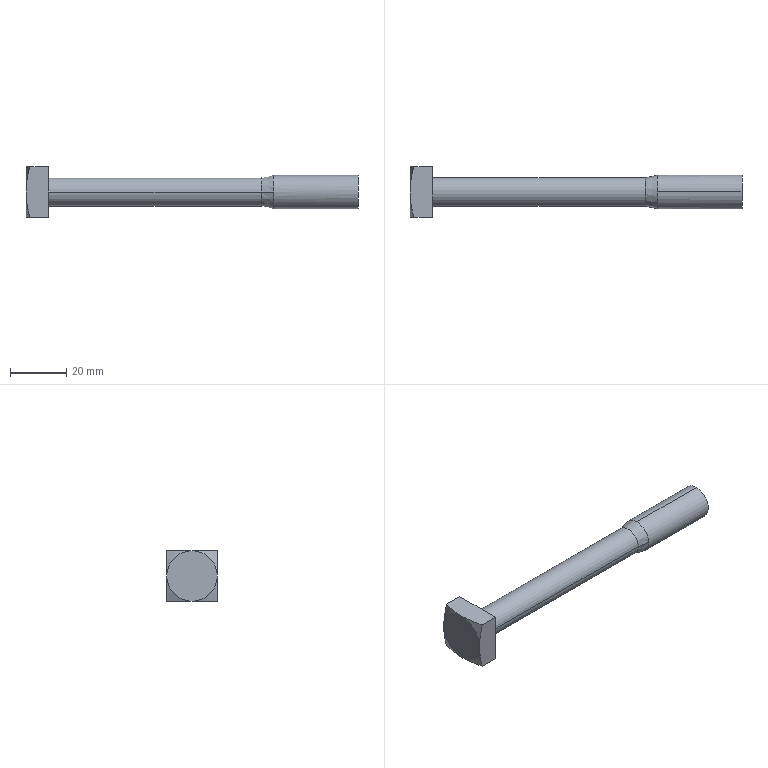Part | SolidWorks | features RevCut 3, Boss 1, Extrusion 1, LPattern 1 | 1 solid | 17 faces | box 118 x 18 x 18 mm | volume 12442 mm3 | plane 7 | cone 6 | cylinder 4 | commonest cylinder face diameters 10.106 x2 12 x2
STEP:
#1=CARTESIAN_POINT('',(118.,0.,-6.));
#2=VERTEX_POINT('',#1);
#3=CARTESIAN_POINT('',(118.,0.,6.));
#4=VERTEX_POINT('',#3);
#5=CARTESIAN_POINT('',(118.,0.,0.));
#6=DIRECTION('',(1.,0.,0.));
#7=DIRECTION('',(0.,0.,-1.));
#8=AXIS2_PLACEMENT_3D('',#5,#6,#7);
#9=CIRCLE('',#8,6.);
#10=EDGE_CURVE('',#2,#4,#9,.T.);
#11=ORIENTED_EDGE('',*,*,#10,.F.);
#12=CARTESIAN_POINT('',(88.,0.,-6.));
#13=VERTEX_POINT('',#12);
#14=CARTESIAN_POINT('',(118.,0.,-6.));
#15=DIRECTION('',(-1.,0.,0.));
#16=VECTOR('',#15,1000.);
#17=LINE('',#14,#16);
#18=EDGE_CURVE('',#2,#13,#17,.T.);
#19=ORIENTED_EDGE('',*,*,#18,.T.);
#20=CARTESIAN_POINT('',(88.,6.,0.));
#21=VERTEX_POINT('',#20);
#22=CARTESIAN_POINT('',(88.,0.,0.));
#23=DIRECTION('',(-1.,0.,0.));
#24=DIRECTION('',(0.,-1.,0.));
#25=AXIS2_PLACEMENT_3D('',#22,#23,#24);
#26=CIRCLE('',#25,6.);
#27=EDGE_CURVE('',#21,#13,#26,.T.);
#28=ORIENTED_EDGE('',*,*,#27,.F.);
#29=CARTESIAN_POINT('',(88.,0.,6.));
#30=VERTEX_POINT('',#29);
#31=CARTESIAN_POINT('',(88.,0.,0.));
#32=DIRECTION('',(-1.,0.,0.));
#33=DIRECTION('',(0.,-1.,0.));
#34=AXIS2_PLACEMENT_3D('',#31,#32,#33);
#35=CIRCLE('',#34,6.);
#36=EDGE_CURVE('',#30,#21,#35,.T.);
#37=ORIENTED_EDGE('',*,*,#36,.F.);
#38=CARTESIAN_POINT('',(118.,0.,6.));
#39=DIRECTION('',(-1.,0.,0.));
#40=VECTOR('',#39,1000.);
#41=LINE('',#38,#40);
#42=EDGE_CURVE('',#4,#30,#41,.T.);
#43=ORIENTED_EDGE('',*,*,#42,.F.);
#44=EDGE_LOOP('',(#11,#19,#28,#37,#43));
#45=FACE_OUTER_BOUND('',#44,.T.);
#46=CARTESIAN_POINT('',(118.,0.,0.));
#47=DIRECTION('',(-1.,0.,0.));
#48=DIRECTION('',(0.,0.,1.));
#49=AXIS2_PLACEMENT_3D('',#46,#47,#48);
#50=CYLINDRICAL_SURFACE('',#49,6.);
#51=ADVANCED_FACE('',(#45),#50,.T.);
#52=CARTESIAN_POINT('',(83.7,-5.053,0.));
#53=VERTEX_POINT('',#52);
#54=CARTESIAN_POINT('',(83.7,5.053,0.));
#55=VERTEX_POINT('',#54);
#56=CARTESIAN_POINT('',(83.7,0.,0.));
#57=DIRECTION('',(-1.,0.,0.));
#58=DIRECTION('',(0.,-1.,0.));
#59=AXIS2_PLACEMENT_3D('',#56,#57,#58);
#60=CIRCLE('',#59,5.053);
#61=EDGE_CURVE('',#53,#55,#60,.T.);
#62=ORIENTED_EDGE('',*,*,#61,.T.);
#63=CARTESIAN_POINT('',(8.,5.053,0.));
#64=VERTEX_POINT('',#63);
#65=CARTESIAN_POINT('',(-3.791,5.053,0.));
#66=DIRECTION('',(-1.,0.,0.));
#67=VECTOR('',#66,1000.);
#68=LINE('',#65,#67);
#69=EDGE_CURVE('',#55,#64,#68,.T.);
#70=ORIENTED_EDGE('',*,*,#69,.T.);
#71=CARTESIAN_POINT('',(8.,-5.053,0.));
#72=VERTEX_POINT('',#71);
#73=CARTESIAN_POINT('',(8.,0.,0.));
#74=DIRECTION('',(-1.,0.,0.));
#75=DIRECTION('',(0.,-1.,0.));
#76=AXIS2_PLACEMENT_3D('',#73,#74,#75);
#77=CIRCLE('',#76,5.053);
#78=EDGE_CURVE('',#72,#64,#77,.T.);
#79=ORIENTED_EDGE('',*,*,#78,.F.);
#80=CARTESIAN_POINT('',(-3.791,-5.053,0.));
#81=DIRECTION('',(-1.,0.,0.));
#82=VECTOR('',#81,1000.);
#83=LINE('',#80,#82);
#84=EDGE_CURVE('',#53,#72,#83,.T.);
#85=ORIENTED_EDGE('',*,*,#84,.F.);
#86=EDGE_LOOP('',(#62,#70,#79,#85));
#87=FACE_OUTER_BOUND('',#86,.T.);
#88=CARTESIAN_POINT('',(-3.791,0.,0.));
#89=DIRECTION('',(-1.,0.,0.));
#90=DIRECTION('',(0.,-1.,0.));
#91=AXIS2_PLACEMENT_3D('',#88,#89,#90);
#92=CYLINDRICAL_SURFACE('',#91,5.053);
#93=ADVANCED_FACE('',(#87),#92,.T.);
#94=ORIENTED_EDGE('',*,*,#61,.F.);
#95=CARTESIAN_POINT('',(88.,-6.,0.));
#96=VERTEX_POINT('',#95);
#97=CARTESIAN_POINT('',(88.,-6.,0.));
#98=DIRECTION('',(0.9766,-0.2151,0.));
#99=VECTOR('',#98,1000.);
#100=LINE('',#97,#99);
#101=EDGE_CURVE('',#53,#96,#100,.T.);
#102=ORIENTED_EDGE('',*,*,#101,.T.);
#103=CARTESIAN_POINT('',(88.,0.,0.));
#104=DIRECTION('',(-1.,0.,0.));
#105=DIRECTION('',(0.,-1.,0.));
#106=AXIS2_PLACEMENT_3D('',#103,#104,#105);
#107=CIRCLE('',#106,6.);
#108=EDGE_CURVE('',#96,#30,#107,.T.);
#109=ORIENTED_EDGE('',*,*,#108,.T.);
#110=ORIENTED_EDGE('',*,*,#36,.T.);
#111=CARTESIAN_POINT('',(88.,6.,0.));
#112=DIRECTION('',(0.9766,0.2151,0.));
#113=VECTOR('',#112,1000.);
#114=LINE('',#111,#113);
#115=EDGE_CURVE('',#55,#21,#114,.T.);
#116=ORIENTED_EDGE('',*,*,#115,.F.);
#117=EDGE_LOOP('',(#94,#102,#109,#110,#116));
#118=FACE_OUTER_BOUND('',#117,.T.);
#119=CARTESIAN_POINT('',(88.,0.,0.));
#120=DIRECTION('',(1.,0.,0.));
#121=DIRECTION('',(0.,1.,0.));
#122=AXIS2_PLACEMENT_3D('',#119,#120,#121);
#123=CONICAL_SURFACE('',#122,6.,0.2168);
#124=ADVANCED_FACE('',(#118),#123,.T.);
#125=CARTESIAN_POINT('',(8.,9.,9.));
#126=VERTEX_POINT('',#125);
#127=CARTESIAN_POINT('',(8.,-9.,9.));
#128=VERTEX_POINT('',#127);
#129=CARTESIAN_POINT('',(8.,9.,9.));
#130=DIRECTION('',(0.,-1.,0.));
#131=VECTOR('',#130,1000.);
#132=LINE('',#129,#131);
#133=EDGE_CURVE('',#126,#128,#132,.T.);
#134=ORIENTED_EDGE('',*,*,#133,.T.);
#135=CARTESIAN_POINT('',(8.,-9.,-9.));
#136=VERTEX_POINT('',#135);
#137=CARTESIAN_POINT('',(8.,-9.,9.));
#138=DIRECTION('',(0.,0.,-1.));
#139=VECTOR('',#138,1000.);
#140=LINE('',#137,#139);
#141=EDGE_CURVE('',#128,#136,#140,.T.);
#142=ORIENTED_EDGE('',*,*,#141,.T.);
#143=CARTESIAN_POINT('',(8.,9.,-9.));
#144=VERTEX_POINT('',#143);
#145=CARTESIAN_POINT('',(8.,9.,-9.));
#146=DIRECTION('',(0.,1.,0.));
#147=VECTOR('',#146,1000.);
#148=LINE('',#145,#147);
#149=EDGE_CURVE('',#136,#144,#148,.T.);
#150=ORIENTED_EDGE('',*,*,#149,.T.);
#151=CARTESIAN_POINT('',(8.,9.,9.));
#152=DIRECTION('',(0.,0.,1.));
#153=VECTOR('',#152,1000.);
#154=LINE('',#151,#153);
#155=EDGE_CURVE('',#144,#126,#154,.T.);
#156=ORIENTED_EDGE('',*,*,#155,.T.);
#157=EDGE_LOOP('',(#134,#142,#150,#156));
#158=FACE_OUTER_BOUND('',#157,.T.);
#159=ORIENTED_EDGE('',*,*,#78,.T.);
#160=CARTESIAN_POINT('',(8.,0.,0.));
#161=DIRECTION('',(-1.,0.,0.));
#162=DIRECTION('',(0.,-1.,0.));
#163=AXIS2_PLACEMENT_3D('',#160,#161,#162);
#164=CIRCLE('',#163,5.053);
#165=EDGE_CURVE('',#64,#72,#164,.T.);
#166=ORIENTED_EDGE('',*,*,#165,.T.);
#167=EDGE_LOOP('',(#159,#166));
#168=FACE_BOUND('',#167,.T.);
#169=CARTESIAN_POINT('',(8.,-9.,9.));
#170=DIRECTION('',(1.,0.,0.));
#171=DIRECTION('',(0.,0.,-1.));
#172=AXIS2_PLACEMENT_3D('',#169,#170,#171);
#173=PLANE('',#172);
#174=ADVANCED_FACE('',(#158,#168),#173,.T.);
#175=CARTESIAN_POINT('',(1.357,-9.,9.));
#176=VERTEX_POINT('',#175);
#177=CARTESIAN_POINT('',(0.,0.,9.));
#178=VERTEX_POINT('',#177);
#179=CARTESIAN_POINT('',(1.357,-9.,9.));
#180=CARTESIAN_POINT('',(0.9754,-7.518,9.));
#181=CARTESIAN_POINT('',(0.6345,-6.018,9.));
#182=CARTESIAN_POINT('',(0.1443,-3.016,9.));
#183=CARTESIAN_POINT('',(0.,-1.511,9.));
#184=CARTESIAN_POINT('',(0.,0.,9.));
#185=B_SPLINE_CURVE_WITH_KNOTS('',3,(#179,#180,#181,#182,#183,#184),.UNSPECIFIED.,.F.,.F.,(4,2,4),(0.009265,0.01385,0.01844),.UNSPECIFIED.);
#186=EDGE_CURVE('',#176,#178,#185,.T.);
#187=ORIENTED_EDGE('',*,*,#186,.F.);
#188=CARTESIAN_POINT('',(8.,-9.,9.));
#189=DIRECTION('',(-1.,0.,0.));
#190=VECTOR('',#189,1000.);
#191=LINE('',#188,#190);
#192=EDGE_CURVE('',#128,#176,#191,.T.);
#193=ORIENTED_EDGE('',*,*,#192,.F.);
#194=ORIENTED_EDGE('',*,*,#133,.F.);
#195=CARTESIAN_POINT('',(1.357,9.,9.));
#196=VERTEX_POINT('',#195);
#197=CARTESIAN_POINT('',(8.,9.,9.));
#198=DIRECTION('',(-1.,0.,0.));
#199=VECTOR('',#198,1000.);
#200=LINE('',#197,#199);
#201=EDGE_CURVE('',#126,#196,#200,.T.);
#202=ORIENTED_EDGE('',*,*,#201,.T.);
#203=CARTESIAN_POINT('',(0.,0.,9.));
#204=CARTESIAN_POINT('',(0.,0.7525,9.));
#205=CARTESIAN_POINT('',(0.03485,1.506,9.));
#206=CARTESIAN_POINT('',(0.1688,3.017,9.));
#207=CARTESIAN_POINT('',(0.2678,3.774,9.));
#208=CARTESIAN_POINT('',(0.6392,6.043,9.));
#209=CARTESIAN_POINT('',(0.978,7.528,9.));
#210=CARTESIAN_POINT('',(1.357,9.,9.));
#211=B_SPLINE_CURVE_WITH_KNOTS('',3,(#203,#204,#205,#206,#207,#208,#209,#210),.UNSPECIFIED.,.F.,.F.,(4,2,2,4),(0.01844,0.02073,0.02302,0.02759),.UNSPECIFIED.);
#212=EDGE_CURVE('',#178,#196,#211,.T.);
#213=ORIENTED_EDGE('',*,*,#212,.F.);
#214=EDGE_LOOP('',(#187,#193,#194,#202,#213));
#215=FACE_OUTER_BOUND('',#214,.T.);
#216=CARTESIAN_POINT('',(8.,9.,9.));
#217=DIRECTION('',(0.,0.,-1.));
#218=DIRECTION('',(-1.,0.,0.));
#219=AXIS2_PLACEMENT_3D('',#216,#217,#218);
#220=PLANE('',#219);
#221=ADVANCED_FACE('',(#215),#220,.F.);
#222=CARTESIAN_POINT('',(1.357,-9.,-9.));
#223=VERTEX_POINT('',#222);
#224=CARTESIAN_POINT('',(0.,-9.,0.));
#225=VERTEX_POINT('',#224);
#226=CARTESIAN_POINT('',(1.357,-9.,-9.));
#227=CARTESIAN_POINT('',(0.9754,-9.,-7.518));
#228=CARTESIAN_POINT('',(0.6345,-9.,-6.018));
#229=CARTESIAN_POINT('',(0.1443,-9.,-3.016));
#230=CARTESIAN_POINT('',(0.,-9.,-1.511));
#231=CARTESIAN_POINT('',(0.,-9.,0.));
#232=B_SPLINE_CURVE_WITH_KNOTS('',3,(#226,#227,#228,#229,#230,#231),.UNSPECIFIED.,.F.,.F.,(4,2,4),(0.009265,0.01385,0.01844),.UNSPECIFIED.);
#233=EDGE_CURVE('',#223,#225,#232,.T.);
#234=ORIENTED_EDGE('',*,*,#233,.F.);
#235=CARTESIAN_POINT('',(8.,-9.,-9.));
#236=DIRECTION('',(-1.,0.,0.));
#237=VECTOR('',#236,1000.);
#238=LINE('',#235,#237);
#239=EDGE_CURVE('',#136,#223,#238,.T.);
#240=ORIENTED_EDGE('',*,*,#239,.F.);
#241=ORIENTED_EDGE('',*,*,#141,.F.);
#242=ORIENTED_EDGE('',*,*,#192,.T.);
#243=CARTESIAN_POINT('',(0.,-9.,0.));
#244=CARTESIAN_POINT('',(0.,-9.,0.7525));
#245=CARTESIAN_POINT('',(0.03485,-9.,1.506));
#246=CARTESIAN_POINT('',(0.1688,-9.,3.017));
#247=CARTESIAN_POINT('',(0.2678,-9.,3.774));
#248=CARTESIAN_POINT('',(0.6392,-9.,6.043));
#249=CARTESIAN_POINT('',(0.978,-9.,7.528));
#250=CARTESIAN_POINT('',(1.357,-9.,9.));
#251=B_SPLINE_CURVE_WITH_KNOTS('',3,(#243,#244,#245,#246,#247,#248,#249,#250),.UNSPECIFIED.,.F.,.F.,(4,2,2,4),(0.01844,0.02073,0.02302,0.02759),.UNSPECIFIED.);
#252=EDGE_CURVE('',#225,#176,#251,.T.);
#253=ORIENTED_EDGE('',*,*,#252,.F.);
#254=EDGE_LOOP('',(#234,#240,#241,#242,#253));
#255=FACE_OUTER_BOUND('',#254,.T.);
#256=CARTESIAN_POINT('',(8.,-9.,9.));
#257=DIRECTION('',(0.,1.,0.));
#258=DIRECTION('',(0.,0.,1.));
#259=AXIS2_PLACEMENT_3D('',#256,#257,#258);
#260=PLANE('',#259);
#261=ADVANCED_FACE('',(#255),#260,.F.);
#262=CARTESIAN_POINT('',(1.357,9.,-9.));
#263=VERTEX_POINT('',#262);
#264=CARTESIAN_POINT('',(0.,0.,-9.));
#265=VERTEX_POINT('',#264);
#266=CARTESIAN_POINT('',(1.357,9.,-9.));
#267=CARTESIAN_POINT('',(0.978,7.528,-9.));
#268=CARTESIAN_POINT('',(0.6392,6.043,-9.));
#269=CARTESIAN_POINT('',(0.2678,3.774,-9.));
#270=CARTESIAN_POINT('',(0.1688,3.017,-9.));
#271=CARTESIAN_POINT('',(0.03485,1.506,-9.));
#272=CARTESIAN_POINT('',(0.,0.7525,-9.));
#273=CARTESIAN_POINT('',(0.,0.,-9.));
#274=B_SPLINE_CURVE_WITH_KNOTS('',3,(#266,#267,#268,#269,#270,#271,#272,#273),.UNSPECIFIED.,.F.,.F.,(4,2,2,4),(0.02832,0.03288,0.03516,0.03743),.UNSPECIFIED.);
#275=EDGE_CURVE('',#263,#265,#274,.T.);
#276=ORIENTED_EDGE('',*,*,#275,.F.);
#277=CARTESIAN_POINT('',(8.,9.,-9.));
#278=DIRECTION('',(-1.,0.,0.));
#279=VECTOR('',#278,1000.);
#280=LINE('',#277,#279);
#281=EDGE_CURVE('',#144,#263,#280,.T.);
#282=ORIENTED_EDGE('',*,*,#281,.F.);
#283=ORIENTED_EDGE('',*,*,#149,.F.);
#284=ORIENTED_EDGE('',*,*,#239,.T.);
#285=CARTESIAN_POINT('',(0.,0.,-9.));
#286=CARTESIAN_POINT('',(0.,-1.511,-9.));
#287=CARTESIAN_POINT('',(0.1443,-3.016,-9.));
#288=CARTESIAN_POINT('',(0.6345,-6.018,-9.));
#289=CARTESIAN_POINT('',(0.9754,-7.518,-9.));
#290=CARTESIAN_POINT('',(1.357,-9.,-9.));
#291=B_SPLINE_CURVE_WITH_KNOTS('',3,(#285,#286,#287,#288,#289,#290),.UNSPECIFIED.,.F.,.F.,(4,2,4),(0.03743,0.042,0.04658),.UNSPECIFIED.);
#292=EDGE_CURVE('',#265,#223,#291,.T.);
#293=ORIENTED_EDGE('',*,*,#292,.F.);
#294=EDGE_LOOP('',(#276,#282,#283,#284,#293));
#295=FACE_OUTER_BOUND('',#294,.T.);
#296=CARTESIAN_POINT('',(8.,9.,-9.));
#297=DIRECTION('',(0.,0.,1.));
#298=DIRECTION('',(0.,-1.,0.));
#299=AXIS2_PLACEMENT_3D('',#296,#297,#298);
#300=PLANE('',#299);
#301=ADVANCED_FACE('',(#295),#300,.F.);
#302=CARTESIAN_POINT('',(0.,9.,0.));
#303=VERTEX_POINT('',#302);
#304=CARTESIAN_POINT('',(1.357,9.,9.));
#305=CARTESIAN_POINT('',(0.978,9.,7.528));
#306=CARTESIAN_POINT('',(0.6392,9.,6.043));
#307=CARTESIAN_POINT('',(0.2678,9.,3.774));
#308=CARTESIAN_POINT('',(0.1688,9.,3.017));
#309=CARTESIAN_POINT('',(0.03485,9.,1.506));
#310=CARTESIAN_POINT('',(0.,9.,0.7525));
#311=CARTESIAN_POINT('',(0.,9.,0.));
#312=B_SPLINE_CURVE_WITH_KNOTS('',3,(#304,#305,#306,#307,#308,#309,#310,#311),.UNSPECIFIED.,.F.,.F.,(4,2,2,4),(0.02832,0.03288,0.03516,0.03743),.UNSPECIFIED.);
#313=EDGE_CURVE('',#196,#303,#312,.T.);
#314=ORIENTED_EDGE('',*,*,#313,.F.);
#315=ORIENTED_EDGE('',*,*,#201,.F.);
#316=ORIENTED_EDGE('',*,*,#155,.F.);
#317=ORIENTED_EDGE('',*,*,#281,.T.);
#318=CARTESIAN_POINT('',(0.,9.,0.));
#319=CARTESIAN_POINT('',(0.,9.,-1.511));
#320=CARTESIAN_POINT('',(0.1443,9.,-3.016));
#321=CARTESIAN_POINT('',(0.6345,9.,-6.018));
#322=CARTESIAN_POINT('',(0.9754,9.,-7.518));
#323=CARTESIAN_POINT('',(1.357,9.,-9.));
#324=B_SPLINE_CURVE_WITH_KNOTS('',3,(#318,#319,#320,#321,#322,#323),.UNSPECIFIED.,.F.,.F.,(4,2,4),(0.03743,0.042,0.04658),.UNSPECIFIED.);
#325=EDGE_CURVE('',#303,#263,#324,.T.);
#326=ORIENTED_EDGE('',*,*,#325,.F.);
#327=EDGE_LOOP('',(#314,#315,#316,#317,#326));
#328=FACE_OUTER_BOUND('',#327,.T.);
#329=CARTESIAN_POINT('',(8.,9.,9.));
#330=DIRECTION('',(0.,-1.,0.));
#331=DIRECTION('',(0.,0.,-1.));
#332=AXIS2_PLACEMENT_3D('',#329,#330,#331);
#333=PLANE('',#332);
#334=ADVANCED_FACE('',(#328),#333,.F.);
#335=ORIENTED_EDGE('',*,*,#233,.T.);
#336=CARTESIAN_POINT('',(0.,0.,0.));
#337=DIRECTION('',(1.,0.,0.));
#338=DIRECTION('',(0.,0.,-1.));
#339=AXIS2_PLACEMENT_3D('',#336,#337,#338);
#340=CIRCLE('',#339,9.);
#341=EDGE_CURVE('',#225,#265,#340,.T.);
#342=ORIENTED_EDGE('',*,*,#341,.T.);
#343=ORIENTED_EDGE('',*,*,#292,.T.);
#344=EDGE_LOOP('',(#335,#342,#343));
#345=FACE_OUTER_BOUND('',#344,.T.);
#346=CARTESIAN_POINT('',(1.357,0.,0.));
#347=DIRECTION('',(1.,0.,0.));
#348=DIRECTION('',(0.,0.,-1.));
#349=AXIS2_PLACEMENT_3D('',#346,#347,#348);
#350=CONICAL_SURFACE('',#349,12.728,1.222);
#351=ADVANCED_FACE('',(#345),#350,.T.);
#352=ORIENTED_EDGE('',*,*,#252,.T.);
#353=ORIENTED_EDGE('',*,*,#186,.T.);
#354=CARTESIAN_POINT('',(0.,0.,0.));
#355=DIRECTION('',(1.,0.,0.));
#356=DIRECTION('',(0.,0.,-1.));
#357=AXIS2_PLACEMENT_3D('',#354,#355,#356);
#358=CIRCLE('',#357,9.);
#359=EDGE_CURVE('',#178,#225,#358,.T.);
#360=ORIENTED_EDGE('',*,*,#359,.T.);
#361=EDGE_LOOP('',(#352,#353,#360));
#362=FACE_OUTER_BOUND('',#361,.T.);
#363=CARTESIAN_POINT('',(1.357,0.,0.));
#364=DIRECTION('',(1.,0.,0.));
#365=DIRECTION('',(0.,0.,-1.));
#366=AXIS2_PLACEMENT_3D('',#363,#364,#365);
#367=CONICAL_SURFACE('',#366,12.728,1.222);
#368=ADVANCED_FACE('',(#362),#367,.T.);
#369=ORIENTED_EDGE('',*,*,#212,.T.);
#370=ORIENTED_EDGE('',*,*,#313,.T.);
#371=CARTESIAN_POINT('',(0.,0.,0.));
#372=DIRECTION('',(1.,0.,0.));
#373=DIRECTION('',(0.,0.,-1.));
#374=AXIS2_PLACEMENT_3D('',#371,#372,#373);
#375=CIRCLE('',#374,9.);
#376=EDGE_CURVE('',#303,#178,#375,.T.);
#377=ORIENTED_EDGE('',*,*,#376,.T.);
#378=EDGE_LOOP('',(#369,#370,#377));
#379=FACE_OUTER_BOUND('',#378,.T.);
#380=CARTESIAN_POINT('',(1.357,0.,0.));
#381=DIRECTION('',(1.,0.,0.));
#382=DIRECTION('',(0.,0.,-1.));
#383=AXIS2_PLACEMENT_3D('',#380,#381,#382);
#384=CONICAL_SURFACE('',#383,12.728,1.222);
#385=ADVANCED_FACE('',(#379),#384,.T.);
#386=ORIENTED_EDGE('',*,*,#275,.T.);
#387=CARTESIAN_POINT('',(0.,0.,0.));
#388=DIRECTION('',(1.,0.,0.));
#389=DIRECTION('',(0.,0.,-1.));
#390=AXIS2_PLACEMENT_3D('',#387,#388,#389);
#391=CIRCLE('',#390,9.);
#392=EDGE_CURVE('',#265,#303,#391,.T.);
#393=ORIENTED_EDGE('',*,*,#392,.T.);
#394=ORIENTED_EDGE('',*,*,#325,.T.);
#395=EDGE_LOOP('',(#386,#393,#394));
#396=FACE_OUTER_BOUND('',#395,.T.);
#397=CARTESIAN_POINT('',(1.357,0.,0.));
#398=DIRECTION('',(1.,0.,0.));
#399=DIRECTION('',(0.,0.,-1.));
#400=AXIS2_PLACEMENT_3D('',#397,#398,#399);
#401=CONICAL_SURFACE('',#400,12.728,1.222);
#402=ADVANCED_FACE('',(#396),#401,.T.);
#403=ORIENTED_EDGE('',*,*,#392,.F.);
#404=ORIENTED_EDGE('',*,*,#341,.F.);
#405=ORIENTED_EDGE('',*,*,#359,.F.);
#406=ORIENTED_EDGE('',*,*,#376,.F.);
#407=EDGE_LOOP('',(#403,#404,#405,#406));
#408=FACE_OUTER_BOUND('',#407,.T.);
#409=CARTESIAN_POINT('',(0.,-9.,9.));
#410=DIRECTION('',(1.,0.,0.));
#411=DIRECTION('',(0.,0.,-1.));
#412=AXIS2_PLACEMENT_3D('',#409,#410,#411);
#413=PLANE('',#412);
#414=ADVANCED_FACE('',(#408),#413,.F.);
#415=ORIENTED_EDGE('',*,*,#101,.F.);
#416=CARTESIAN_POINT('',(83.7,0.,0.));
#417=DIRECTION('',(-1.,0.,0.));
#418=DIRECTION('',(0.,-1.,0.));
#419=AXIS2_PLACEMENT_3D('',#416,#417,#418);
#420=CIRCLE('',#419,5.053);
#421=EDGE_CURVE('',#55,#53,#420,.T.);
#422=ORIENTED_EDGE('',*,*,#421,.F.);
#423=ORIENTED_EDGE('',*,*,#115,.T.);
#424=ORIENTED_EDGE('',*,*,#27,.T.);
#425=CARTESIAN_POINT('',(88.,0.,0.));
#426=DIRECTION('',(-1.,0.,0.));
#427=DIRECTION('',(0.,-1.,0.));
#428=AXIS2_PLACEMENT_3D('',#425,#426,#427);
#429=CIRCLE('',#428,6.);
#430=EDGE_CURVE('',#13,#96,#429,.T.);
#431=ORIENTED_EDGE('',*,*,#430,.T.);
#432=EDGE_LOOP('',(#415,#422,#423,#424,#431));
#433=FACE_OUTER_BOUND('',#432,.T.);
#434=CARTESIAN_POINT('',(88.,0.,0.));
#435=DIRECTION('',(1.,0.,0.));
#436=DIRECTION('',(0.,1.,0.));
#437=AXIS2_PLACEMENT_3D('',#434,#435,#436);
#438=CONICAL_SURFACE('',#437,6.,0.2168);
#439=ADVANCED_FACE('',(#433),#438,.T.);
#440=ORIENTED_EDGE('',*,*,#69,.F.);
#441=ORIENTED_EDGE('',*,*,#421,.T.);
#442=ORIENTED_EDGE('',*,*,#84,.T.);
#443=ORIENTED_EDGE('',*,*,#165,.F.);
#444=EDGE_LOOP('',(#440,#441,#442,#443));
#445=FACE_OUTER_BOUND('',#444,.T.);
#446=CARTESIAN_POINT('',(-3.791,0.,0.));
#447=DIRECTION('',(-1.,0.,0.));
#448=DIRECTION('',(0.,-1.,0.));
#449=AXIS2_PLACEMENT_3D('',#446,#447,#448);
#450=CYLINDRICAL_SURFACE('',#449,5.053);
#451=ADVANCED_FACE('',(#445),#450,.T.);
#452=CARTESIAN_POINT('',(118.,0.,0.));
#453=DIRECTION('',(1.,0.,0.));
#454=DIRECTION('',(0.,0.,-1.));
#455=AXIS2_PLACEMENT_3D('',#452,#453,#454);
#456=CIRCLE('',#455,6.);
#457=EDGE_CURVE('',#4,#2,#456,.T.);
#458=ORIENTED_EDGE('',*,*,#457,.T.);
#459=ORIENTED_EDGE('',*,*,#10,.T.);
#460=EDGE_LOOP('',(#458,#459));
#461=FACE_OUTER_BOUND('',#460,.T.);
#462=CARTESIAN_POINT('',(118.,0.,0.));
#463=DIRECTION('',(1.,0.,0.));
#464=DIRECTION('',(0.,0.,-1.));
#465=AXIS2_PLACEMENT_3D('',#462,#463,#464);
#466=PLANE('',#465);
#467=ADVANCED_FACE('',(#461),#466,.T.);
#468=ORIENTED_EDGE('',*,*,#18,.F.);
#469=ORIENTED_EDGE('',*,*,#457,.F.);
#470=ORIENTED_EDGE('',*,*,#42,.T.);
#471=ORIENTED_EDGE('',*,*,#108,.F.);
#472=ORIENTED_EDGE('',*,*,#430,.F.);
#473=EDGE_LOOP('',(#468,#469,#470,#471,#472));
#474=FACE_OUTER_BOUND('',#473,.T.);
#475=CARTESIAN_POINT('',(118.,0.,0.));
#476=DIRECTION('',(-1.,0.,0.));
#477=DIRECTION('',(0.,0.,1.));
#478=AXIS2_PLACEMENT_3D('',#475,#476,#477);
#479=CYLINDRICAL_SURFACE('',#478,6.);
#480=ADVANCED_FACE('',(#474),#479,.T.);
#481=CLOSED_SHELL('',(#51,#93,#124,#174,#221,#261,#301,#334,#351,#368,#385,#402,#414,#439,#451,#467,#480));
#482=MANIFOLD_SOLID_BREP('',#481);
#483=CARTESIAN_POINT('',(0.,0.,0.));
#484=DIRECTION('',(0.,0.,1.));
#485=DIRECTION('',(1.,0.,0.));
#486=AXIS2_PLACEMENT_3D('',#483,#484,#485);
#487=(LENGTH_UNIT()NAMED_UNIT(*)SI_UNIT(.MILLI.,.METRE.));
#488=UNCERTAINTY_MEASURE_WITH_UNIT(LENGTH_MEASURE(0.00001),#487,'','');
#489=(NAMED_UNIT(*)PLANE_ANGLE_UNIT()SI_UNIT($,.RADIAN.));
#490=(NAMED_UNIT(*)SI_UNIT($,.STERADIAN.)SOLID_ANGLE_UNIT());
#491=(GEOMETRIC_REPRESENTATION_CONTEXT(3)GLOBAL_UNCERTAINTY_ASSIGNED_CONTEXT((#488))GLOBAL_UNIT_ASSIGNED_CONTEXT((#487,#489,#490))REPRESENTATION_CONTEXT('',''));
#492=ADVANCED_BREP_SHAPE_REPRESENTATION('',(#482,#486),#491);